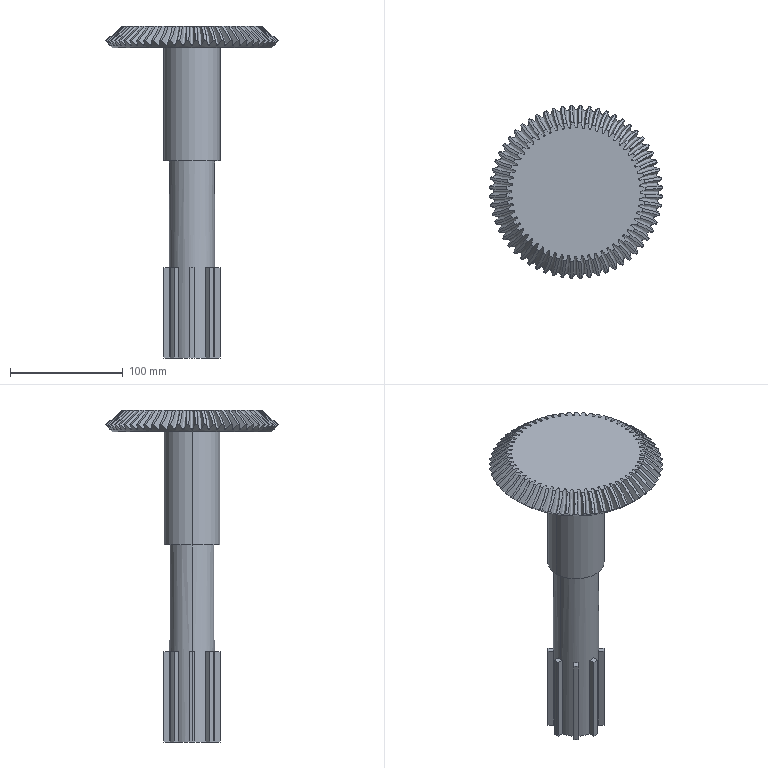Part | SolidWorks | 1 solid | 163 faces | box 153.486 x 153.486 x 294.64 mm | volume 719014 mm3 | cone 62 | spline 60 | plane 28 | cylinder 13 | commonest cylinder face diameters 50 x11 40 x2